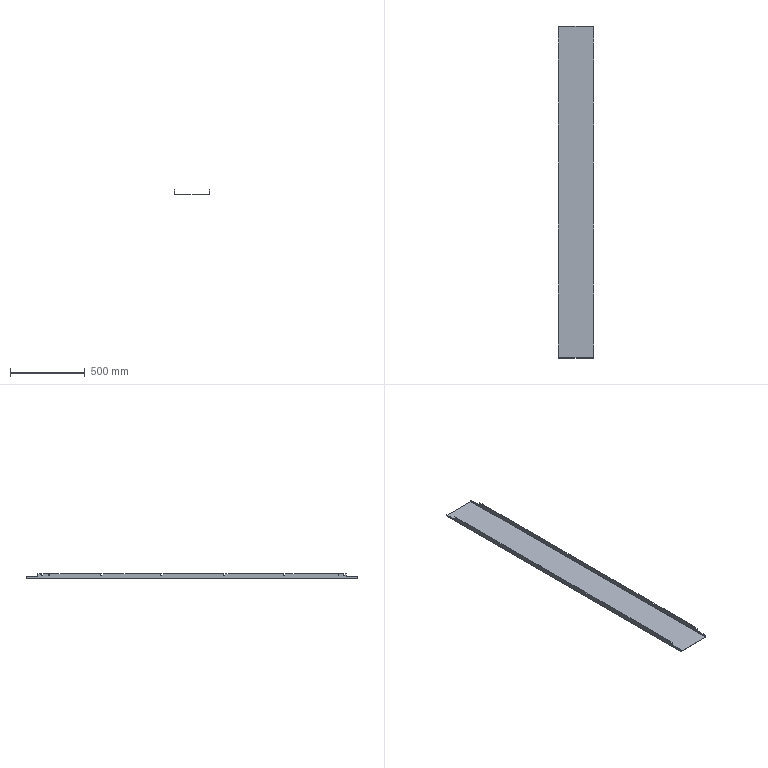Part | SolidWorks | features ICE 4, Chamfer 2, Fillet 1, FlatPattern 1, SMBaseFlange 1, SheetMetal 1 | 1 solid | 102 faces | box 235 x 2216 x 33 mm | volume 782016 mm3 | plane 66 | cylinder 36 | commonest cylinder face diameters 8.2 x24 6 x8 0.4 x2 2.8 x2